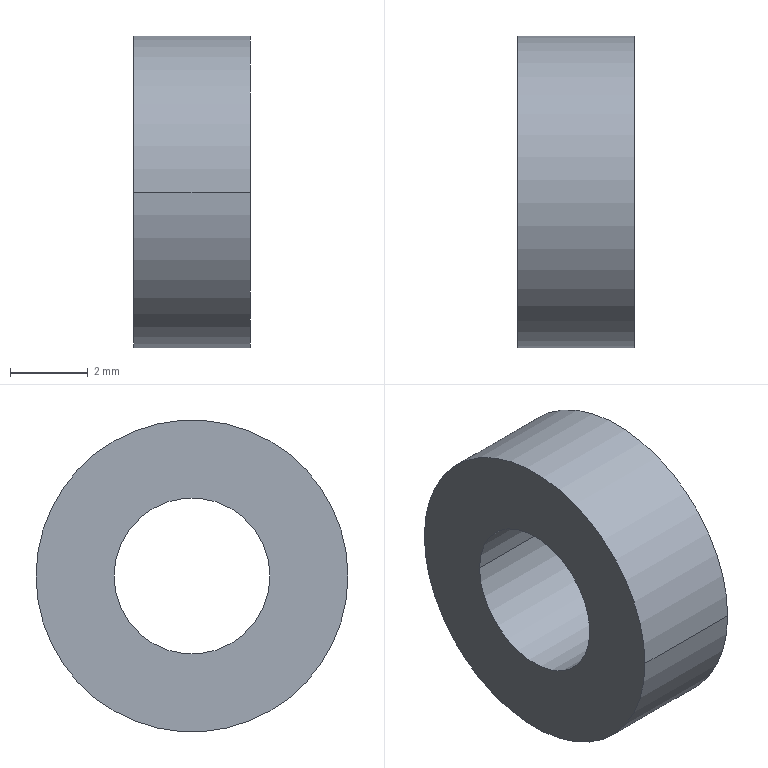Part | STEP file | 0246_004_WSJJ8-4-3 | 1 solid | 6 faces | box 3 x 8 x 8 mm | volume 113.097 mm3 | cylinder 4 | plane 2 | commonest cylinder face diameters 4 x2 8 x2
STEP:
#1=CARTESIAN_POINT('',(0.,0.,0.));
#2=DIRECTION('',(0.,0.,1.));
#3=DIRECTION('',(1.,0.,0.));
#4=AXIS2_PLACEMENT_3D('',#1,#2,#3);
#5=CARTESIAN_POINT('',(3.,-4.,0.));
#6=VERTEX_POINT('',#5);
#7=CARTESIAN_POINT('',(3.,4.,0.));
#8=VERTEX_POINT('',#7);
#9=CARTESIAN_POINT('',(3.,0.,0.));
#10=DIRECTION('',(-1.,0.,0.));
#11=DIRECTION('',(0.,-1.,0.));
#12=AXIS2_PLACEMENT_3D('',#9,#10,#11);
#13=CIRCLE('',#12,4.);
#14=CARTESIAN_POINT('',(1.5,0.,0.));
#15=DIRECTION('',(-1.,0.,0.));
#16=DIRECTION('',(0.,-1.,0.));
#17=AXIS2_PLACEMENT_3D('',#14,#15,#16);
#18=CYLINDRICAL_SURFACE('',#17,4.);
#19=CARTESIAN_POINT('',(0.,-1.5));
#20=DIRECTION('',(1.,0.));
#21=VECTOR('',#20,1.);
#22=LINE('',#19,#21);
#23=(GEOMETRIC_REPRESENTATION_CONTEXT(2)PARAMETRIC_REPRESENTATION_CONTEXT()REPRESENTATION_CONTEXT('',''));
#24=DEFINITIONAL_REPRESENTATION('',(#22),#23);
#25=PCURVE('',#18,#24);
#26=CARTESIAN_POINT('',(3.,-3.,0.));
#27=DIRECTION('',(1.,0.,0.));
#28=DIRECTION('',(0.,1.,0.));
#29=AXIS2_PLACEMENT_3D('',#26,#27,#28);
#30=PLANE('',#29);
#31=CARTESIAN_POINT('',(-1.,0.));
#32=CARTESIAN_POINT('',(-1.,6.928));
#33=CARTESIAN_POINT('',(5.,3.464));
#34=CARTESIAN_POINT('',(11.,0.));
#35=CARTESIAN_POINT('',(5.,-3.464));
#36=CARTESIAN_POINT('',(-1.,-6.928));
#37=CARTESIAN_POINT('',(-1.,0.));
#38=(BOUNDED_CURVE()B_SPLINE_CURVE(2,(#31,#32,#33,#34,#35,#36,#37),.UNSPECIFIED.,.T.,.F.)B_SPLINE_CURVE_WITH_KNOTS((1,2,2,2,2,1),(-2.094,0.,2.094,4.189,6.283,8.378),.UNSPECIFIED.)CURVE()GEOMETRIC_REPRESENTATION_ITEM()RATIONAL_B_SPLINE_CURVE((1.,0.5,1.,0.5,1.,0.5,1.))REPRESENTATION_ITEM(''));
#39=(GEOMETRIC_REPRESENTATION_CONTEXT(2)PARAMETRIC_REPRESENTATION_CONTEXT()REPRESENTATION_CONTEXT('',''));
#40=DEFINITIONAL_REPRESENTATION('',(#38),#39);
#41=PCURVE('',#30,#40);
#42=SURFACE_CURVE('',#13,(#25,#41),.PCURVE_S1.);
#43=EDGE_CURVE('',#6,#8,#42,.T.);
#44=ORIENTED_EDGE('',*,*,#43,.T.);
#45=CARTESIAN_POINT('',(0.,4.,0.));
#46=VERTEX_POINT('',#45);
#47=CARTESIAN_POINT('',(1.5,4.,0.));
#48=DIRECTION('',(-1.,0.,0.));
#49=VECTOR('',#48,1.);
#50=LINE('',#47,#49);
#51=CARTESIAN_POINT('',(3.142,0.));
#52=DIRECTION('',(0.,1.));
#53=VECTOR('',#52,1.);
#54=LINE('',#51,#53);
#55=(GEOMETRIC_REPRESENTATION_CONTEXT(2)PARAMETRIC_REPRESENTATION_CONTEXT()REPRESENTATION_CONTEXT('',''));
#56=DEFINITIONAL_REPRESENTATION('',(#54),#55);
#57=PCURVE('',#18,#56);
#58=CARTESIAN_POINT('',(1.5,0.,0.));
#59=DIRECTION('',(-1.,0.,0.));
#60=DIRECTION('',(0.,-1.,0.));
#61=AXIS2_PLACEMENT_3D('',#58,#59,#60);
#62=CYLINDRICAL_SURFACE('',#61,4.);
#63=CARTESIAN_POINT('',(3.142,0.));
#64=DIRECTION('',(0.,1.));
#65=VECTOR('',#64,1.);
#66=LINE('',#63,#65);
#67=(GEOMETRIC_REPRESENTATION_CONTEXT(2)PARAMETRIC_REPRESENTATION_CONTEXT()REPRESENTATION_CONTEXT('',''));
#68=DEFINITIONAL_REPRESENTATION('',(#66),#67);
#69=PCURVE('',#62,#68);
#70=SURFACE_CURVE('',#50,(#57,#69),.PCURVE_S1.);
#71=EDGE_CURVE('',#8,#46,#70,.T.);
#72=ORIENTED_EDGE('',*,*,#71,.T.);
#73=CARTESIAN_POINT('',(0.,-4.,0.));
#74=VERTEX_POINT('',#73);
#75=CARTESIAN_POINT('',(0.,0.,0.));
#76=DIRECTION('',(1.,0.,0.));
#77=DIRECTION('',(0.,-1.,0.));
#78=AXIS2_PLACEMENT_3D('',#75,#76,#77);
#79=CIRCLE('',#78,4.);
#80=CARTESIAN_POINT('',(6.283,1.5));
#81=DIRECTION('',(-1.,0.));
#82=VECTOR('',#81,1.);
#83=LINE('',#80,#82);
#84=(GEOMETRIC_REPRESENTATION_CONTEXT(2)PARAMETRIC_REPRESENTATION_CONTEXT()REPRESENTATION_CONTEXT('',''));
#85=DEFINITIONAL_REPRESENTATION('',(#83),#84);
#86=PCURVE('',#18,#85);
#87=CARTESIAN_POINT('',(0.,-3.,0.));
#88=DIRECTION('',(-1.,0.,0.));
#89=DIRECTION('',(0.,-1.,0.));
#90=AXIS2_PLACEMENT_3D('',#87,#88,#89);
#91=PLANE('',#90);
#92=CARTESIAN_POINT('',(1.,0.));
#93=CARTESIAN_POINT('',(1.,-6.928));
#94=CARTESIAN_POINT('',(-5.,-3.464));
#95=CARTESIAN_POINT('',(-11.,0.));
#96=CARTESIAN_POINT('',(-5.,3.464));
#97=CARTESIAN_POINT('',(1.,6.928));
#98=CARTESIAN_POINT('',(1.,0.));
#99=(BOUNDED_CURVE()B_SPLINE_CURVE(2,(#92,#93,#94,#95,#96,#97,#98),.UNSPECIFIED.,.T.,.F.)B_SPLINE_CURVE_WITH_KNOTS((1,2,2,2,2,1),(-2.094,0.,2.094,4.189,6.283,8.378),.UNSPECIFIED.)CURVE()GEOMETRIC_REPRESENTATION_ITEM()RATIONAL_B_SPLINE_CURVE((1.,0.5,1.,0.5,1.,0.5,1.))REPRESENTATION_ITEM(''));
#100=(GEOMETRIC_REPRESENTATION_CONTEXT(2)PARAMETRIC_REPRESENTATION_CONTEXT()REPRESENTATION_CONTEXT('',''));
#101=DEFINITIONAL_REPRESENTATION('',(#99),#100);
#102=PCURVE('',#91,#101);
#103=SURFACE_CURVE('',#79,(#86,#102),.PCURVE_S1.);
#104=EDGE_CURVE('',#46,#74,#103,.T.);
#105=ORIENTED_EDGE('',*,*,#104,.T.);
#106=CARTESIAN_POINT('',(1.5,-4.,0.));
#107=DIRECTION('',(-1.,0.,0.));
#108=VECTOR('',#107,1.);
#109=LINE('',#106,#108);
#110=CARTESIAN_POINT('',(0.,0.));
#111=DIRECTION('',(0.,1.));
#112=VECTOR('',#111,1.);
#113=LINE('',#110,#112);
#114=(GEOMETRIC_REPRESENTATION_CONTEXT(2)PARAMETRIC_REPRESENTATION_CONTEXT()REPRESENTATION_CONTEXT('',''));
#115=DEFINITIONAL_REPRESENTATION('',(#113),#114);
#116=PCURVE('',#18,#115);
#117=CARTESIAN_POINT('',(6.283,0.));
#118=DIRECTION('',(0.,1.));
#119=VECTOR('',#118,1.);
#120=LINE('',#117,#119);
#121=(GEOMETRIC_REPRESENTATION_CONTEXT(2)PARAMETRIC_REPRESENTATION_CONTEXT()REPRESENTATION_CONTEXT('',''));
#122=DEFINITIONAL_REPRESENTATION('',(#120),#121);
#123=PCURVE('',#62,#122);
#124=SURFACE_CURVE('',#109,(#116,#123),.PCURVE_S1.);
#125=EDGE_CURVE('',#6,#74,#124,.T.);
#126=ORIENTED_EDGE('',*,*,#125,.F.);
#127=EDGE_LOOP('',(#44,#72,#105,#126));
#128=FACE_BOUND('',#127,.T.);
#129=ADVANCED_FACE('',(#128),#18,.T.);
#130=CARTESIAN_POINT('',(3.,-2.,0.));
#131=VERTEX_POINT('',#130);
#132=CARTESIAN_POINT('',(0.,-2.,0.));
#133=VERTEX_POINT('',#132);
#134=CARTESIAN_POINT('',(1.5,-2.,0.));
#135=DIRECTION('',(-1.,0.,0.));
#136=VECTOR('',#135,1.);
#137=LINE('',#134,#136);
#138=CARTESIAN_POINT('',(1.5,0.,0.));
#139=DIRECTION('',(-1.,0.,0.));
#140=DIRECTION('',(0.,-1.,0.));
#141=AXIS2_PLACEMENT_3D('',#138,#139,#140);
#142=CYLINDRICAL_SURFACE('',#141,2.);
#143=CARTESIAN_POINT('',(6.283,0.));
#144=DIRECTION('',(0.,1.));
#145=VECTOR('',#144,1.);
#146=LINE('',#143,#145);
#147=(GEOMETRIC_REPRESENTATION_CONTEXT(2)PARAMETRIC_REPRESENTATION_CONTEXT()REPRESENTATION_CONTEXT('',''));
#148=DEFINITIONAL_REPRESENTATION('',(#146),#147);
#149=PCURVE('',#142,#148);
#150=CARTESIAN_POINT('',(1.5,0.,0.));
#151=DIRECTION('',(-1.,0.,0.));
#152=DIRECTION('',(0.,-1.,0.));
#153=AXIS2_PLACEMENT_3D('',#150,#151,#152);
#154=CYLINDRICAL_SURFACE('',#153,2.);
#155=CARTESIAN_POINT('',(0.,0.));
#156=DIRECTION('',(0.,1.));
#157=VECTOR('',#156,1.);
#158=LINE('',#155,#157);
#159=(GEOMETRIC_REPRESENTATION_CONTEXT(2)PARAMETRIC_REPRESENTATION_CONTEXT()REPRESENTATION_CONTEXT('',''));
#160=DEFINITIONAL_REPRESENTATION('',(#158),#159);
#161=PCURVE('',#154,#160);
#162=SURFACE_CURVE('',#137,(#149,#161),.PCURVE_S1.);
#163=EDGE_CURVE('',#131,#133,#162,.T.);
#164=ORIENTED_EDGE('',*,*,#163,.T.);
#165=CARTESIAN_POINT('',(0.,2.,0.));
#166=VERTEX_POINT('',#165);
#167=CARTESIAN_POINT('',(0.,0.,0.));
#168=DIRECTION('',(1.,0.,0.));
#169=DIRECTION('',(0.,-1.,0.));
#170=AXIS2_PLACEMENT_3D('',#167,#168,#169);
#171=CIRCLE('',#170,2.);
#172=CARTESIAN_POINT('',(6.283,1.5));
#173=DIRECTION('',(-1.,0.));
#174=VECTOR('',#173,1.);
#175=LINE('',#172,#174);
#176=(GEOMETRIC_REPRESENTATION_CONTEXT(2)PARAMETRIC_REPRESENTATION_CONTEXT()REPRESENTATION_CONTEXT('',''));
#177=DEFINITIONAL_REPRESENTATION('',(#175),#176);
#178=PCURVE('',#142,#177);
#179=CARTESIAN_POINT('',(-1.,0.));
#180=CARTESIAN_POINT('',(-1.,-3.464));
#181=CARTESIAN_POINT('',(-4.,-1.732));
#182=CARTESIAN_POINT('',(-7.,0.));
#183=CARTESIAN_POINT('',(-4.,1.732));
#184=CARTESIAN_POINT('',(-1.,3.464));
#185=CARTESIAN_POINT('',(-1.,0.));
#186=(BOUNDED_CURVE()B_SPLINE_CURVE(2,(#179,#180,#181,#182,#183,#184,#185),.UNSPECIFIED.,.T.,.F.)B_SPLINE_CURVE_WITH_KNOTS((1,2,2,2,2,1),(-2.094,0.,2.094,4.189,6.283,8.378),.UNSPECIFIED.)CURVE()GEOMETRIC_REPRESENTATION_ITEM()RATIONAL_B_SPLINE_CURVE((1.,0.5,1.,0.5,1.,0.5,1.))REPRESENTATION_ITEM(''));
#187=(GEOMETRIC_REPRESENTATION_CONTEXT(2)PARAMETRIC_REPRESENTATION_CONTEXT()REPRESENTATION_CONTEXT('',''));
#188=DEFINITIONAL_REPRESENTATION('',(#186),#187);
#189=PCURVE('',#91,#188);
#190=SURFACE_CURVE('',#171,(#178,#189),.PCURVE_S1.);
#191=EDGE_CURVE('',#133,#166,#190,.T.);
#192=ORIENTED_EDGE('',*,*,#191,.T.);
#193=CARTESIAN_POINT('',(3.,2.,0.));
#194=VERTEX_POINT('',#193);
#195=CARTESIAN_POINT('',(1.5,2.,0.));
#196=DIRECTION('',(-1.,0.,0.));
#197=VECTOR('',#196,1.);
#198=LINE('',#195,#197);
#199=CARTESIAN_POINT('',(3.142,0.));
#200=DIRECTION('',(0.,1.));
#201=VECTOR('',#200,1.);
#202=LINE('',#199,#201);
#203=(GEOMETRIC_REPRESENTATION_CONTEXT(2)PARAMETRIC_REPRESENTATION_CONTEXT()REPRESENTATION_CONTEXT('',''));
#204=DEFINITIONAL_REPRESENTATION('',(#202),#203);
#205=PCURVE('',#142,#204);
#206=CARTESIAN_POINT('',(3.142,0.));
#207=DIRECTION('',(0.,1.));
#208=VECTOR('',#207,1.);
#209=LINE('',#206,#208);
#210=(GEOMETRIC_REPRESENTATION_CONTEXT(2)PARAMETRIC_REPRESENTATION_CONTEXT()REPRESENTATION_CONTEXT('',''));
#211=DEFINITIONAL_REPRESENTATION('',(#209),#210);
#212=PCURVE('',#154,#211);
#213=SURFACE_CURVE('',#198,(#205,#212),.PCURVE_S1.);
#214=EDGE_CURVE('',#194,#166,#213,.T.);
#215=ORIENTED_EDGE('',*,*,#214,.F.);
#216=CARTESIAN_POINT('',(3.,0.,0.));
#217=DIRECTION('',(-1.,0.,0.));
#218=DIRECTION('',(0.,-1.,0.));
#219=AXIS2_PLACEMENT_3D('',#216,#217,#218);
#220=CIRCLE('',#219,2.);
#221=CARTESIAN_POINT('',(0.,-1.5));
#222=DIRECTION('',(1.,0.));
#223=VECTOR('',#222,1.);
#224=LINE('',#221,#223);
#225=(GEOMETRIC_REPRESENTATION_CONTEXT(2)PARAMETRIC_REPRESENTATION_CONTEXT()REPRESENTATION_CONTEXT('',''));
#226=DEFINITIONAL_REPRESENTATION('',(#224),#225);
#227=PCURVE('',#142,#226);
#228=CARTESIAN_POINT('',(1.,0.));
#229=CARTESIAN_POINT('',(1.,3.464));
#230=CARTESIAN_POINT('',(4.,1.732));
#231=CARTESIAN_POINT('',(7.,0.));
#232=CARTESIAN_POINT('',(4.,-1.732));
#233=CARTESIAN_POINT('',(1.,-3.464));
#234=CARTESIAN_POINT('',(1.,0.));
#235=(BOUNDED_CURVE()B_SPLINE_CURVE(2,(#228,#229,#230,#231,#232,#233,#234),.UNSPECIFIED.,.T.,.F.)B_SPLINE_CURVE_WITH_KNOTS((1,2,2,2,2,1),(-2.094,0.,2.094,4.189,6.283,8.378),.UNSPECIFIED.)CURVE()GEOMETRIC_REPRESENTATION_ITEM()RATIONAL_B_SPLINE_CURVE((1.,0.5,1.,0.5,1.,0.5,1.))REPRESENTATION_ITEM(''));
#236=(GEOMETRIC_REPRESENTATION_CONTEXT(2)PARAMETRIC_REPRESENTATION_CONTEXT()REPRESENTATION_CONTEXT('',''));
#237=DEFINITIONAL_REPRESENTATION('',(#235),#236);
#238=PCURVE('',#30,#237);
#239=SURFACE_CURVE('',#220,(#227,#238),.PCURVE_S1.);
#240=EDGE_CURVE('',#194,#131,#239,.T.);
#241=ORIENTED_EDGE('',*,*,#240,.T.);
#242=EDGE_LOOP('',(#164,#192,#215,#241));
#243=FACE_BOUND('',#242,.F.);
#244=ADVANCED_FACE('',(#243),#142,.F.);
#245=ORIENTED_EDGE('',*,*,#71,.F.);
#246=CARTESIAN_POINT('',(3.,0.,0.));
#247=DIRECTION('',(-1.,0.,0.));
#248=DIRECTION('',(0.,-1.,0.));
#249=AXIS2_PLACEMENT_3D('',#246,#247,#248);
#250=CIRCLE('',#249,4.);
#251=CARTESIAN_POINT('',(0.,-1.5));
#252=DIRECTION('',(1.,0.));
#253=VECTOR('',#252,1.);
#254=LINE('',#251,#253);
#255=(GEOMETRIC_REPRESENTATION_CONTEXT(2)PARAMETRIC_REPRESENTATION_CONTEXT()REPRESENTATION_CONTEXT('',''));
#256=DEFINITIONAL_REPRESENTATION('',(#254),#255);
#257=PCURVE('',#62,#256);
#258=CARTESIAN_POINT('',(-1.,0.));
#259=CARTESIAN_POINT('',(-1.,6.928));
#260=CARTESIAN_POINT('',(5.,3.464));
#261=CARTESIAN_POINT('',(11.,0.));
#262=CARTESIAN_POINT('',(5.,-3.464));
#263=CARTESIAN_POINT('',(-1.,-6.928));
#264=CARTESIAN_POINT('',(-1.,0.));
#265=(BOUNDED_CURVE()B_SPLINE_CURVE(2,(#258,#259,#260,#261,#262,#263,#264),.UNSPECIFIED.,.T.,.F.)B_SPLINE_CURVE_WITH_KNOTS((1,2,2,2,2,1),(-2.094,0.,2.094,4.189,6.283,8.378),.UNSPECIFIED.)CURVE()GEOMETRIC_REPRESENTATION_ITEM()RATIONAL_B_SPLINE_CURVE((1.,0.5,1.,0.5,1.,0.5,1.))REPRESENTATION_ITEM(''));
#266=(GEOMETRIC_REPRESENTATION_CONTEXT(2)PARAMETRIC_REPRESENTATION_CONTEXT()REPRESENTATION_CONTEXT('',''));
#267=DEFINITIONAL_REPRESENTATION('',(#265),#266);
#268=PCURVE('',#30,#267);
#269=SURFACE_CURVE('',#250,(#257,#268),.PCURVE_S1.);
#270=EDGE_CURVE('',#8,#6,#269,.T.);
#271=ORIENTED_EDGE('',*,*,#270,.T.);
#272=ORIENTED_EDGE('',*,*,#125,.T.);
#273=CARTESIAN_POINT('',(0.,0.,0.));
#274=DIRECTION('',(1.,0.,0.));
#275=DIRECTION('',(0.,-1.,0.));
#276=AXIS2_PLACEMENT_3D('',#273,#274,#275);
#277=CIRCLE('',#276,4.);
#278=CARTESIAN_POINT('',(6.283,1.5));
#279=DIRECTION('',(-1.,0.));
#280=VECTOR('',#279,1.);
#281=LINE('',#278,#280);
#282=(GEOMETRIC_REPRESENTATION_CONTEXT(2)PARAMETRIC_REPRESENTATION_CONTEXT()REPRESENTATION_CONTEXT('',''));
#283=DEFINITIONAL_REPRESENTATION('',(#281),#282);
#284=PCURVE('',#62,#283);
#285=CARTESIAN_POINT('',(1.,0.));
#286=CARTESIAN_POINT('',(1.,-6.928));
#287=CARTESIAN_POINT('',(-5.,-3.464));
#288=CARTESIAN_POINT('',(-11.,0.));
#289=CARTESIAN_POINT('',(-5.,3.464));
#290=CARTESIAN_POINT('',(1.,6.928));
#291=CARTESIAN_POINT('',(1.,0.));
#292=(BOUNDED_CURVE()B_SPLINE_CURVE(2,(#285,#286,#287,#288,#289,#290,#291),.UNSPECIFIED.,.T.,.F.)B_SPLINE_CURVE_WITH_KNOTS((1,2,2,2,2,1),(-2.094,0.,2.094,4.189,6.283,8.378),.UNSPECIFIED.)CURVE()GEOMETRIC_REPRESENTATION_ITEM()RATIONAL_B_SPLINE_CURVE((1.,0.5,1.,0.5,1.,0.5,1.))REPRESENTATION_ITEM(''));
#293=(GEOMETRIC_REPRESENTATION_CONTEXT(2)PARAMETRIC_REPRESENTATION_CONTEXT()REPRESENTATION_CONTEXT('',''));
#294=DEFINITIONAL_REPRESENTATION('',(#292),#293);
#295=PCURVE('',#91,#294);
#296=SURFACE_CURVE('',#277,(#284,#295),.PCURVE_S1.);
#297=EDGE_CURVE('',#74,#46,#296,.T.);
#298=ORIENTED_EDGE('',*,*,#297,.T.);
#299=EDGE_LOOP('',(#245,#271,#272,#298));
#300=FACE_BOUND('',#299,.T.);
#301=ADVANCED_FACE('',(#300),#62,.T.);
#302=ORIENTED_EDGE('',*,*,#43,.F.);
#303=ORIENTED_EDGE('',*,*,#270,.F.);
#304=EDGE_LOOP('',(#302,#303));
#305=FACE_BOUND('',#304,.T.);
#306=CARTESIAN_POINT('',(3.,0.,0.));
#307=DIRECTION('',(-1.,0.,0.));
#308=DIRECTION('',(0.,-1.,0.));
#309=AXIS2_PLACEMENT_3D('',#306,#307,#308);
#310=CIRCLE('',#309,2.);
#311=CARTESIAN_POINT('',(1.,0.));
#312=CARTESIAN_POINT('',(1.,3.464));
#313=CARTESIAN_POINT('',(4.,1.732));
#314=CARTESIAN_POINT('',(7.,0.));
#315=CARTESIAN_POINT('',(4.,-1.732));
#316=CARTESIAN_POINT('',(1.,-3.464));
#317=CARTESIAN_POINT('',(1.,0.));
#318=(BOUNDED_CURVE()B_SPLINE_CURVE(2,(#311,#312,#313,#314,#315,#316,#317),.UNSPECIFIED.,.T.,.F.)B_SPLINE_CURVE_WITH_KNOTS((1,2,2,2,2,1),(-2.094,0.,2.094,4.189,6.283,8.378),.UNSPECIFIED.)CURVE()GEOMETRIC_REPRESENTATION_ITEM()RATIONAL_B_SPLINE_CURVE((1.,0.5,1.,0.5,1.,0.5,1.))REPRESENTATION_ITEM(''));
#319=(GEOMETRIC_REPRESENTATION_CONTEXT(2)PARAMETRIC_REPRESENTATION_CONTEXT()REPRESENTATION_CONTEXT('',''));
#320=DEFINITIONAL_REPRESENTATION('',(#318),#319);
#321=PCURVE('',#30,#320);
#322=CARTESIAN_POINT('',(0.,-1.5));
#323=DIRECTION('',(1.,0.));
#324=VECTOR('',#323,1.);
#325=LINE('',#322,#324);
#326=(GEOMETRIC_REPRESENTATION_CONTEXT(2)PARAMETRIC_REPRESENTATION_CONTEXT()REPRESENTATION_CONTEXT('',''));
#327=DEFINITIONAL_REPRESENTATION('',(#325),#326);
#328=PCURVE('',#154,#327);
#329=SURFACE_CURVE('',#310,(#321,#328),.PCURVE_S1.);
#330=EDGE_CURVE('',#131,#194,#329,.T.);
#331=ORIENTED_EDGE('',*,*,#330,.T.);
#332=ORIENTED_EDGE('',*,*,#240,.T.);
#333=EDGE_LOOP('',(#331,#332));
#334=FACE_BOUND('',#333,.T.);
#335=ADVANCED_FACE('',(#305,#334),#30,.T.);
#336=ORIENTED_EDGE('',*,*,#191,.T.);
#337=CARTESIAN_POINT('',(0.,0.,0.));
#338=DIRECTION('',(1.,0.,0.));
#339=DIRECTION('',(0.,-1.,0.));
#340=AXIS2_PLACEMENT_3D('',#337,#338,#339);
#341=CIRCLE('',#340,2.);
#342=CARTESIAN_POINT('',(-1.,0.));
#343=CARTESIAN_POINT('',(-1.,-3.464));
#344=CARTESIAN_POINT('',(-4.,-1.732));
#345=CARTESIAN_POINT('',(-7.,0.));
#346=CARTESIAN_POINT('',(-4.,1.732));
#347=CARTESIAN_POINT('',(-1.,3.464));
#348=CARTESIAN_POINT('',(-1.,0.));
#349=(BOUNDED_CURVE()B_SPLINE_CURVE(2,(#342,#343,#344,#345,#346,#347,#348),.UNSPECIFIED.,.T.,.F.)B_SPLINE_CURVE_WITH_KNOTS((1,2,2,2,2,1),(-2.094,0.,2.094,4.189,6.283,8.378),.UNSPECIFIED.)CURVE()GEOMETRIC_REPRESENTATION_ITEM()RATIONAL_B_SPLINE_CURVE((1.,0.5,1.,0.5,1.,0.5,1.))REPRESENTATION_ITEM(''));
#350=(GEOMETRIC_REPRESENTATION_CONTEXT(2)PARAMETRIC_REPRESENTATION_CONTEXT()REPRESENTATION_CONTEXT('',''));
#351=DEFINITIONAL_REPRESENTATION('',(#349),#350);
#352=PCURVE('',#91,#351);
#353=CARTESIAN_POINT('',(6.283,1.5));
#354=DIRECTION('',(-1.,0.));
#355=VECTOR('',#354,1.);
#356=LINE('',#353,#355);
#357=(GEOMETRIC_REPRESENTATION_CONTEXT(2)PARAMETRIC_REPRESENTATION_CONTEXT()REPRESENTATION_CONTEXT('',''));
#358=DEFINITIONAL_REPRESENTATION('',(#356),#357);
#359=PCURVE('',#154,#358);
#360=SURFACE_CURVE('',#341,(#352,#359),.PCURVE_S1.);
#361=EDGE_CURVE('',#166,#133,#360,.T.);
#362=ORIENTED_EDGE('',*,*,#361,.T.);
#363=EDGE_LOOP('',(#336,#362));
#364=FACE_BOUND('',#363,.T.);
#365=ORIENTED_EDGE('',*,*,#297,.F.);
#366=ORIENTED_EDGE('',*,*,#104,.F.);
#367=EDGE_LOOP('',(#365,#366));
#368=FACE_BOUND('',#367,.T.);
#369=ADVANCED_FACE('',(#364,#368),#91,.T.);
#370=ORIENTED_EDGE('',*,*,#361,.T.);
#371=ORIENTED_EDGE('',*,*,#163,.F.);
#372=ORIENTED_EDGE('',*,*,#330,.T.);
#373=ORIENTED_EDGE('',*,*,#214,.T.);
#374=EDGE_LOOP('',(#370,#371,#372,#373));
#375=FACE_BOUND('',#374,.F.);
#376=ADVANCED_FACE('',(#375),#154,.F.);
#377=CLOSED_SHELL('',(#129,#244,#301,#335,#369,#376));
#378=MANIFOLD_SOLID_BREP('',#377);
#379=(LENGTH_UNIT()NAMED_UNIT(*)SI_UNIT(.MILLI.,.METRE.));
#380=UNCERTAINTY_MEASURE_WITH_UNIT(LENGTH_MEASURE(0.0000001),#379,'','');
#381=(NAMED_UNIT(*)PLANE_ANGLE_UNIT()SI_UNIT($,.RADIAN.));
#382=(NAMED_UNIT(*)SI_UNIT($,.STERADIAN.)SOLID_ANGLE_UNIT());
#383=(GEOMETRIC_REPRESENTATION_CONTEXT(3)GLOBAL_UNCERTAINTY_ASSIGNED_CONTEXT((#380))GLOBAL_UNIT_ASSIGNED_CONTEXT((#379,#381,#382))REPRESENTATION_CONTEXT('',''));
#384=ADVANCED_BREP_SHAPE_REPRESENTATION('',(#4,#378),#383);